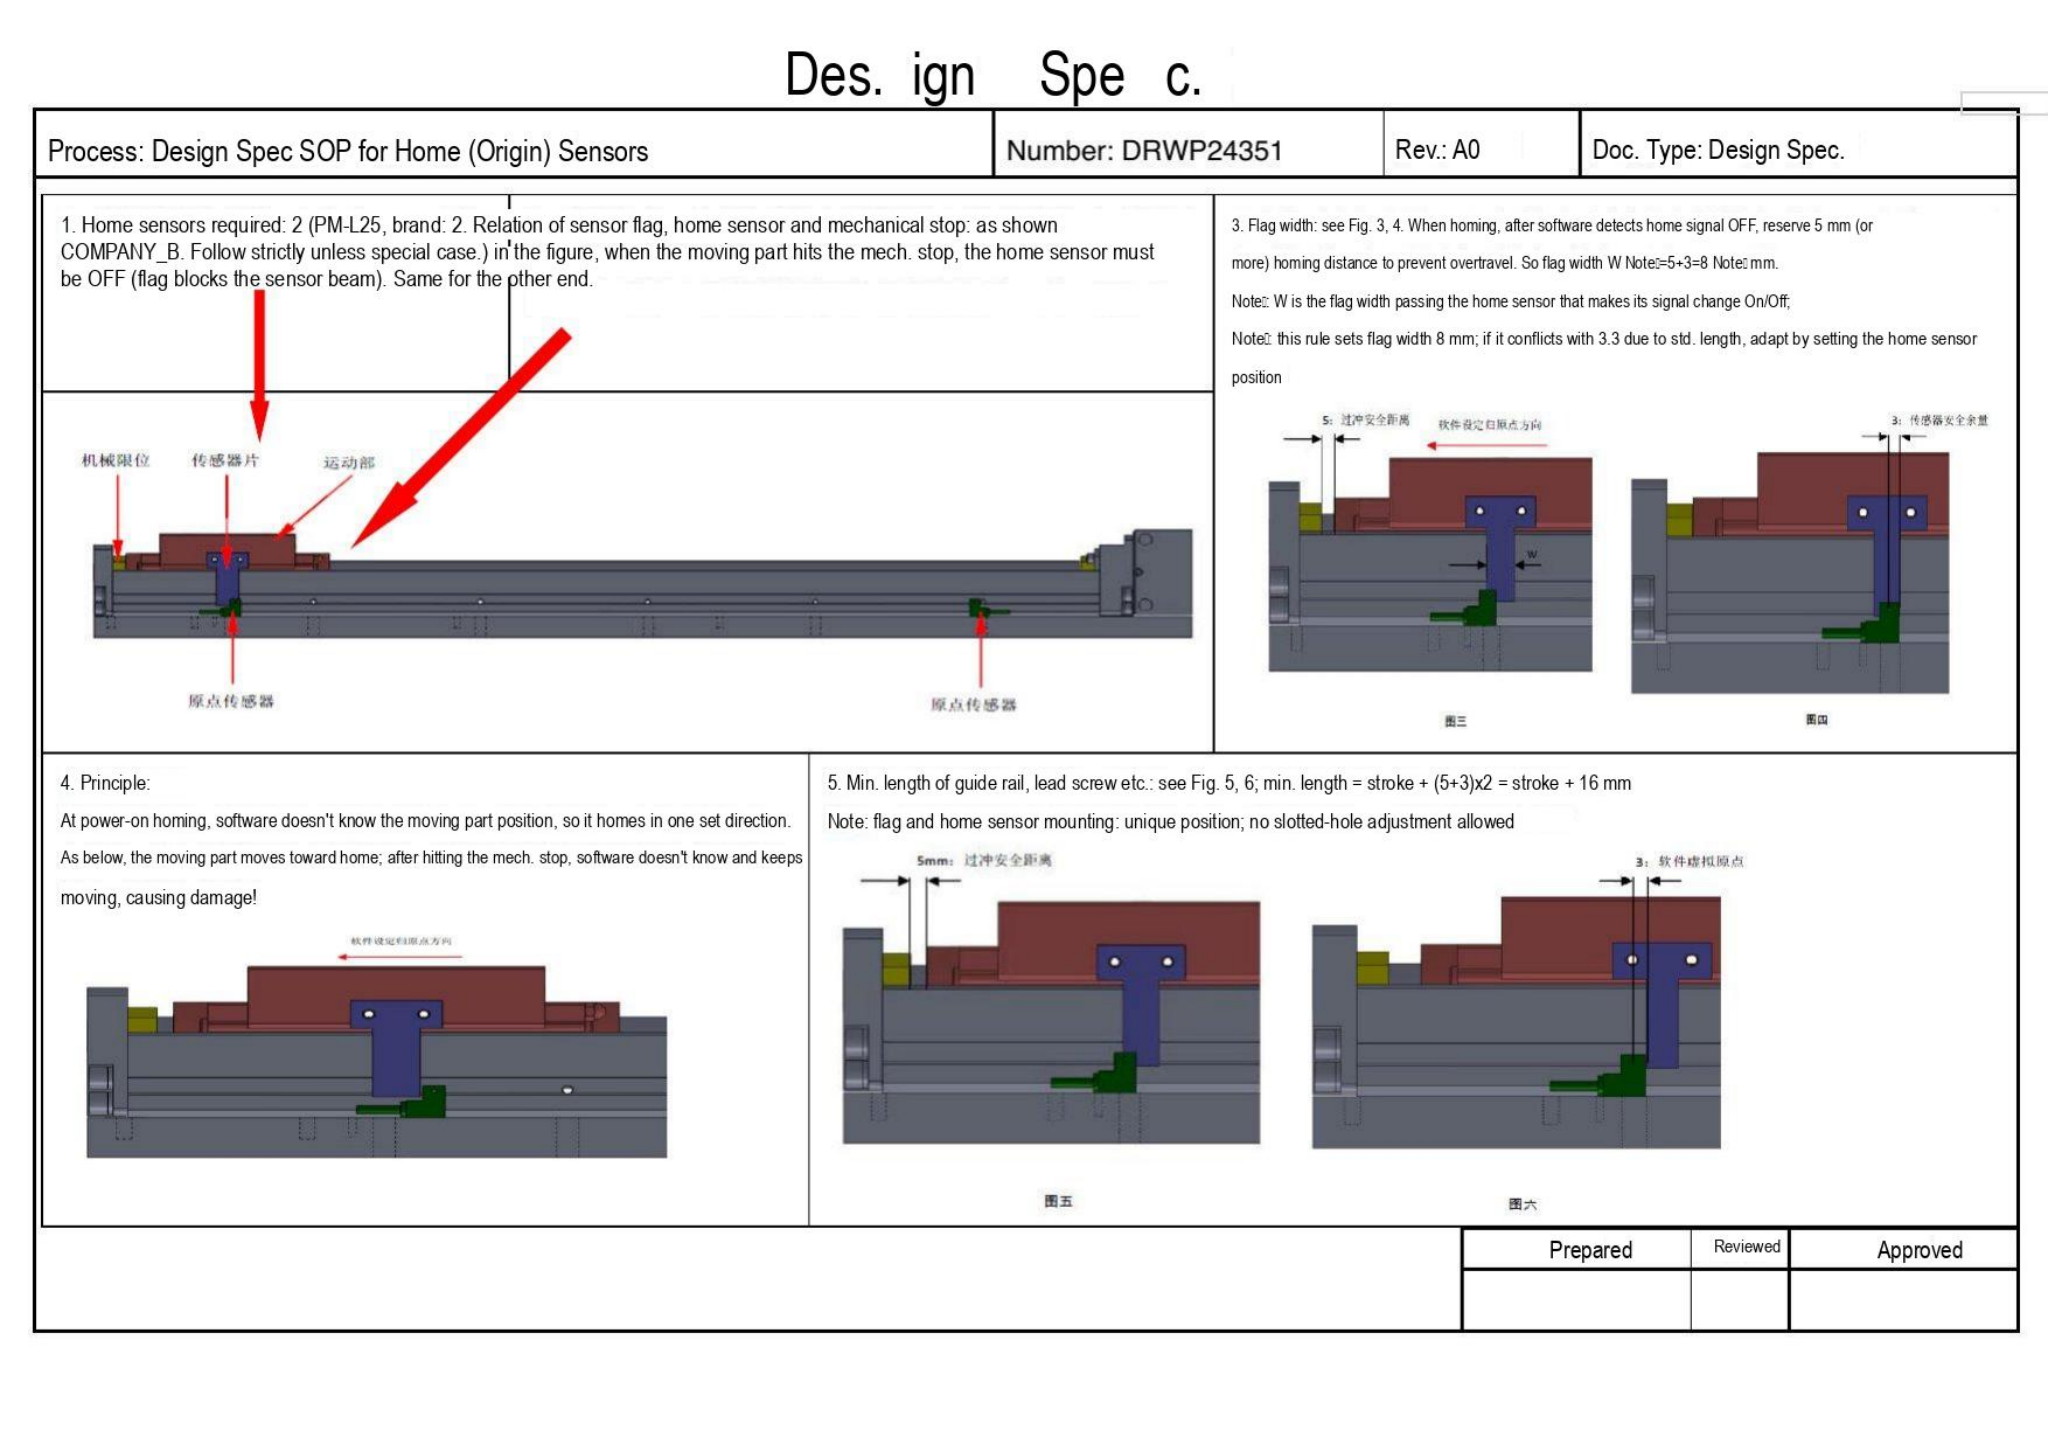Des. ign Spe c.

| Process: Design Spec SOP for Home (Origin) Sensors | Number: DRWP24351 | Rev.: A0 | Doc. Type: Design Spec. |
|---|---|---|---|

1. Home sensors required: 2 (PM-L25, brand: COMPANY_B. Follow strictly unless special case.)

2. Relation of sensor flag, home sensor and mechanical stop: as shown in the figure, when the moving part hits the mech. stop, the home sensor must be OFF (flag blocks the sensor beam). Same for the other end.

机械限位 传感器片 运动部

原点传感器 原点传感器

3. Flag width: see Fig. 3, 4. When homing, after software detects home signal OFF, reserve 5 mm (or more) homing distance to prevent overtravel. So flag width W Note□=5+3=8 Note□ mm.

Note□: W is the flag width passing the home sensor that makes its signal change On/Off;

Note□: this rule sets flag width 8 mm; if it conflicts with 3.3 due to std. length, adapt by setting the home sensor position

5: 过冲安全距离 软件设定归原点方向 W 3: 传感器安全余量

图三 图四

4. Principle:

At power-on homing, software doesn't know the moving part position, so it homes in one set direction.

As below, the moving part moves toward home; after hitting the mech. stop, software doesn't know and keeps moving, causing damage!

软件设定归原点方向

5. Min. length of guide rail, lead screw etc.: see Fig. 5, 6; min. length = stroke + (5+3)x2 = stroke + 16 mm

Note: flag and home sensor mounting: unique position; no slotted-hole adjustment allowed

5mm: 过冲安全距离 3: 软件虚拟原点

图五 图六

| Prepared | Reviewed | Approved |
|---|---|---|
| | | |